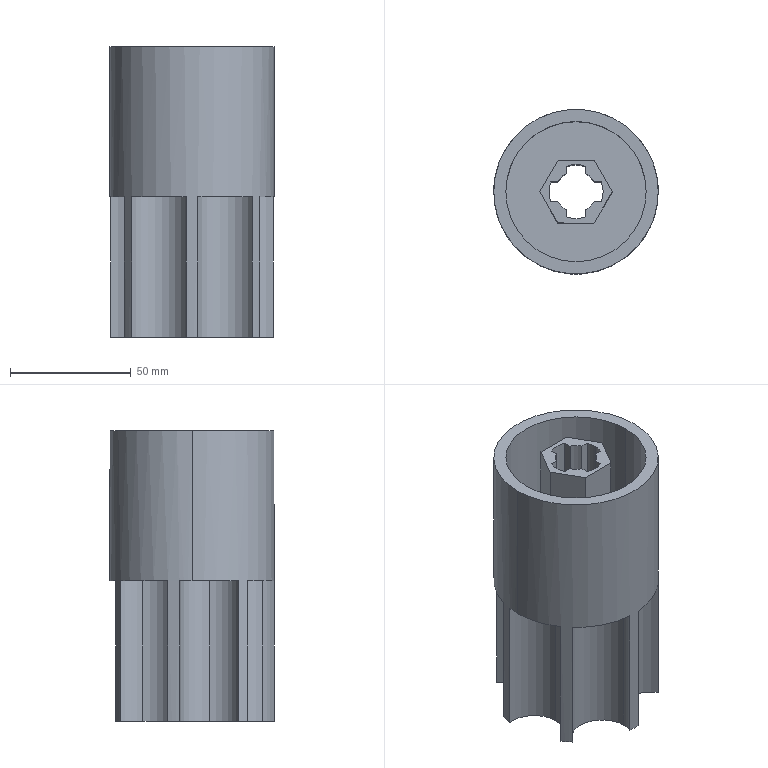Part | SolidWorks | features ICE 2, Extrusion 1 | 1 solid | 48 faces | box 68 x 68 x 120 mm | volume 167321 mm3 | plane 25 | cylinder 23 | commonest cylinder face diameters 25.067 x10 22.4 x5 17 x4 58 x2 68 x2
STEP:
#1=CARTESIAN_POINT('',(11.2,0.,-60.));
#2=VERTEX_POINT('',#1);
#3=CARTESIAN_POINT('',(10.461,4.,-60.));
#4=VERTEX_POINT('',#3);
#5=CARTESIAN_POINT('',(0.,0.,-60.));
#6=DIRECTION('',(0.,0.,1.));
#7=DIRECTION('',(1.,0.,0.));
#8=AXIS2_PLACEMENT_3D('',#5,#6,#7);
#9=CIRCLE('',#8,11.2);
#10=EDGE_CURVE('',#2,#4,#9,.T.);
#11=ORIENTED_EDGE('',*,*,#10,.F.);
#12=CARTESIAN_POINT('',(11.2,0.,60.));
#13=VERTEX_POINT('',#12);
#14=CARTESIAN_POINT('',(11.2,0.,-60.));
#15=DIRECTION('',(0.,0.,1.));
#16=VECTOR('',#15,1000.);
#17=LINE('',#14,#16);
#18=EDGE_CURVE('',#2,#13,#17,.T.);
#19=ORIENTED_EDGE('',*,*,#18,.T.);
#20=CARTESIAN_POINT('',(10.461,4.,60.));
#21=VERTEX_POINT('',#20);
#22=CARTESIAN_POINT('',(0.,0.,60.));
#23=DIRECTION('',(0.,0.,1.));
#24=DIRECTION('',(1.,0.,0.));
#25=AXIS2_PLACEMENT_3D('',#22,#23,#24);
#26=CIRCLE('',#25,11.2);
#27=EDGE_CURVE('',#13,#21,#26,.T.);
#28=ORIENTED_EDGE('',*,*,#27,.T.);
#29=CARTESIAN_POINT('',(10.461,4.,-60.));
#30=DIRECTION('',(0.,0.,1.));
#31=VECTOR('',#30,1000.);
#32=LINE('',#29,#31);
#33=EDGE_CURVE('',#4,#21,#32,.T.);
#34=ORIENTED_EDGE('',*,*,#33,.F.);
#35=EDGE_LOOP('',(#11,#19,#28,#34));
#36=FACE_OUTER_BOUND('',#35,.T.);
#37=CARTESIAN_POINT('',(0.,0.,-60.));
#38=DIRECTION('',(0.,0.,1.));
#39=DIRECTION('',(1.,0.,0.));
#40=AXIS2_PLACEMENT_3D('',#37,#38,#39);
#41=CYLINDRICAL_SURFACE('',#40,11.2);
#42=ADVANCED_FACE('',(#36),#41,.F.);
#43=CARTESIAN_POINT('',(34.,0.,60.));
#44=VERTEX_POINT('',#43);
#45=CARTESIAN_POINT('',(-34.,0.,60.));
#46=VERTEX_POINT('',#45);
#47=CARTESIAN_POINT('',(0.,0.,60.));
#48=DIRECTION('',(0.,0.,1.));
#49=DIRECTION('',(1.,0.,0.));
#50=AXIS2_PLACEMENT_3D('',#47,#48,#49);
#51=CIRCLE('',#50,34.);
#52=EDGE_CURVE('',#44,#46,#51,.T.);
#53=ORIENTED_EDGE('',*,*,#52,.F.);
#54=CARTESIAN_POINT('',(34.,0.,-2.));
#55=VERTEX_POINT('',#54);
#56=CARTESIAN_POINT('',(34.,0.,60.));
#57=DIRECTION('',(0.,0.,-1.));
#58=VECTOR('',#57,1000.);
#59=LINE('',#56,#58);
#60=EDGE_CURVE('',#44,#55,#59,.T.);
#61=ORIENTED_EDGE('',*,*,#60,.T.);
#62=CARTESIAN_POINT('',(33.608,5.151,-2.));
#63=VERTEX_POINT('',#62);
#64=CARTESIAN_POINT('',(0.,0.,-2.));
#65=DIRECTION('',(0.,0.,1.));
#66=DIRECTION('',(1.,0.,0.));
#67=AXIS2_PLACEMENT_3D('',#64,#65,#66);
#68=CIRCLE('',#67,34.);
#69=EDGE_CURVE('',#55,#63,#68,.T.);
#70=ORIENTED_EDGE('',*,*,#69,.T.);
#71=CARTESIAN_POINT('',(33.608,5.151,-60.));
#72=VERTEX_POINT('',#71);
#73=CARTESIAN_POINT('',(33.608,5.151,-60.));
#74=DIRECTION('',(0.,0.,1.));
#75=VECTOR('',#74,1000.);
#76=LINE('',#73,#75);
#77=EDGE_CURVE('',#72,#63,#76,.T.);
#78=ORIENTED_EDGE('',*,*,#77,.F.);
#79=CARTESIAN_POINT('',(32.514,9.941,-60.));
#80=VERTEX_POINT('',#79);
#81=CARTESIAN_POINT('',(0.,0.,-60.));
#82=DIRECTION('',(0.,0.,1.));
#83=DIRECTION('',(1.,0.,0.));
#84=AXIS2_PLACEMENT_3D('',#81,#82,#83);
#85=CIRCLE('',#84,34.);
#86=EDGE_CURVE('',#72,#80,#85,.T.);
#87=ORIENTED_EDGE('',*,*,#86,.T.);
#88=CARTESIAN_POINT('',(32.514,9.941,-2.));
#89=VERTEX_POINT('',#88);
#90=CARTESIAN_POINT('',(32.514,9.941,-60.));
#91=DIRECTION('',(0.,0.,1.));
#92=VECTOR('',#91,1000.);
#93=LINE('',#90,#92);
#94=EDGE_CURVE('',#80,#89,#93,.T.);
#95=ORIENTED_EDGE('',*,*,#94,.T.);
#96=CARTESIAN_POINT('',(16.927,29.487,-2.));
#97=VERTEX_POINT('',#96);
#98=CARTESIAN_POINT('',(0.,0.,-2.));
#99=DIRECTION('',(0.,0.,1.));
#100=DIRECTION('',(1.,0.,0.));
#101=AXIS2_PLACEMENT_3D('',#98,#99,#100);
#102=CIRCLE('',#101,34.);
#103=EDGE_CURVE('',#89,#97,#102,.T.);
#104=ORIENTED_EDGE('',*,*,#103,.T.);
#105=CARTESIAN_POINT('',(16.927,29.487,-60.));
#106=VERTEX_POINT('',#105);
#107=CARTESIAN_POINT('',(16.927,29.487,-60.));
#108=DIRECTION('',(0.,0.,1.));
#109=VECTOR('',#108,1000.);
#110=LINE('',#107,#109);
#111=EDGE_CURVE('',#106,#97,#110,.T.);
#112=ORIENTED_EDGE('',*,*,#111,.F.);
#113=CARTESIAN_POINT('',(12.5,31.619,-60.));
#114=VERTEX_POINT('',#113);
#115=CARTESIAN_POINT('',(0.,0.,-60.));
#116=DIRECTION('',(0.,0.,1.));
#117=DIRECTION('',(1.,0.,0.));
#118=AXIS2_PLACEMENT_3D('',#115,#116,#117);
#119=CIRCLE('',#118,34.);
#120=EDGE_CURVE('',#106,#114,#119,.T.);
#121=ORIENTED_EDGE('',*,*,#120,.T.);
#122=CARTESIAN_POINT('',(12.5,31.619,-2.));
#123=VERTEX_POINT('',#122);
#124=CARTESIAN_POINT('',(12.5,31.619,-60.));
#125=DIRECTION('',(0.,0.,1.));
#126=VECTOR('',#125,1000.);
#127=LINE('',#124,#126);
#128=EDGE_CURVE('',#114,#123,#127,.T.);
#129=ORIENTED_EDGE('',*,*,#128,.T.);
#130=CARTESIAN_POINT('',(-12.5,31.619,-2.));
#131=VERTEX_POINT('',#130);
#132=CARTESIAN_POINT('',(0.,0.,-2.));
#133=DIRECTION('',(0.,0.,1.));
#134=DIRECTION('',(1.,0.,0.));
#135=AXIS2_PLACEMENT_3D('',#132,#133,#134);
#136=CIRCLE('',#135,34.);
#137=EDGE_CURVE('',#123,#131,#136,.T.);
#138=ORIENTED_EDGE('',*,*,#137,.T.);
#139=CARTESIAN_POINT('',(-12.5,31.619,-60.));
#140=VERTEX_POINT('',#139);
#141=CARTESIAN_POINT('',(-12.5,31.619,-60.));
#142=DIRECTION('',(0.,0.,1.));
#143=VECTOR('',#142,1000.);
#144=LINE('',#141,#143);
#145=EDGE_CURVE('',#140,#131,#144,.T.);
#146=ORIENTED_EDGE('',*,*,#145,.F.);
#147=CARTESIAN_POINT('',(-16.927,29.487,-60.));
#148=VERTEX_POINT('',#147);
#149=CARTESIAN_POINT('',(0.,0.,-60.));
#150=DIRECTION('',(0.,0.,1.));
#151=DIRECTION('',(1.,0.,0.));
#152=AXIS2_PLACEMENT_3D('',#149,#150,#151);
#153=CIRCLE('',#152,34.);
#154=EDGE_CURVE('',#140,#148,#153,.T.);
#155=ORIENTED_EDGE('',*,*,#154,.T.);
#156=CARTESIAN_POINT('',(-16.927,29.487,-2.));
#157=VERTEX_POINT('',#156);
#158=CARTESIAN_POINT('',(-16.927,29.487,-60.));
#159=DIRECTION('',(0.,0.,1.));
#160=VECTOR('',#159,1000.);
#161=LINE('',#158,#160);
#162=EDGE_CURVE('',#148,#157,#161,.T.);
#163=ORIENTED_EDGE('',*,*,#162,.T.);
#164=CARTESIAN_POINT('',(-32.514,9.941,-2.));
#165=VERTEX_POINT('',#164);
#166=CARTESIAN_POINT('',(0.,0.,-2.));
#167=DIRECTION('',(0.,0.,1.));
#168=DIRECTION('',(1.,0.,0.));
#169=AXIS2_PLACEMENT_3D('',#166,#167,#168);
#170=CIRCLE('',#169,34.);
#171=EDGE_CURVE('',#157,#165,#170,.T.);
#172=ORIENTED_EDGE('',*,*,#171,.T.);
#173=CARTESIAN_POINT('',(-32.514,9.941,-60.));
#174=VERTEX_POINT('',#173);
#175=CARTESIAN_POINT('',(-32.514,9.941,-60.));
#176=DIRECTION('',(0.,0.,1.));
#177=VECTOR('',#176,1000.);
#178=LINE('',#175,#177);
#179=EDGE_CURVE('',#174,#165,#178,.T.);
#180=ORIENTED_EDGE('',*,*,#179,.F.);
#181=CARTESIAN_POINT('',(-33.608,5.151,-60.));
#182=VERTEX_POINT('',#181);
#183=CARTESIAN_POINT('',(0.,0.,-60.));
#184=DIRECTION('',(0.,0.,1.));
#185=DIRECTION('',(1.,0.,0.));
#186=AXIS2_PLACEMENT_3D('',#183,#184,#185);
#187=CIRCLE('',#186,34.);
#188=EDGE_CURVE('',#174,#182,#187,.T.);
#189=ORIENTED_EDGE('',*,*,#188,.T.);
#190=CARTESIAN_POINT('',(-33.608,5.151,-2.));
#191=VERTEX_POINT('',#190);
#192=CARTESIAN_POINT('',(-33.608,5.151,-60.));
#193=DIRECTION('',(0.,0.,1.));
#194=VECTOR('',#193,1000.);
#195=LINE('',#192,#194);
#196=EDGE_CURVE('',#182,#191,#195,.T.);
#197=ORIENTED_EDGE('',*,*,#196,.T.);
#198=CARTESIAN_POINT('',(-34.,0.,-2.));
#199=VERTEX_POINT('',#198);
#200=CARTESIAN_POINT('',(0.,0.,-2.));
#201=DIRECTION('',(0.,0.,1.));
#202=DIRECTION('',(1.,0.,0.));
#203=AXIS2_PLACEMENT_3D('',#200,#201,#202);
#204=CIRCLE('',#203,34.);
#205=EDGE_CURVE('',#191,#199,#204,.T.);
#206=ORIENTED_EDGE('',*,*,#205,.T.);
#207=CARTESIAN_POINT('',(-34.,0.,60.));
#208=DIRECTION('',(0.,0.,-1.));
#209=VECTOR('',#208,1000.);
#210=LINE('',#207,#209);
#211=EDGE_CURVE('',#46,#199,#210,.T.);
#212=ORIENTED_EDGE('',*,*,#211,.F.);
#213=EDGE_LOOP('',(#53,#61,#70,#78,#87,#95,#104,#112,#121,#129,#138,#146,#155,#163,#172,#180,#189,#197,#206,#212));
#214=FACE_OUTER_BOUND('',#213,.T.);
#215=CARTESIAN_POINT('',(0.,0.,60.));
#216=DIRECTION('',(0.,0.,-1.));
#217=DIRECTION('',(-1.,0.,0.));
#218=AXIS2_PLACEMENT_3D('',#215,#216,#217);
#219=CYLINDRICAL_SURFACE('',#218,34.);
#220=ADVANCED_FACE('',(#214),#219,.T.);
#221=CARTESIAN_POINT('',(-29.,0.,60.));
#222=VERTEX_POINT('',#221);
#223=CARTESIAN_POINT('',(29.,0.,60.));
#224=VERTEX_POINT('',#223);
#225=CARTESIAN_POINT('',(0.,0.,60.));
#226=DIRECTION('',(0.,0.,1.));
#227=DIRECTION('',(1.,0.,0.));
#228=AXIS2_PLACEMENT_3D('',#225,#226,#227);
#229=CIRCLE('',#228,29.);
#230=EDGE_CURVE('',#222,#224,#229,.T.);
#231=ORIENTED_EDGE('',*,*,#230,.T.);
#232=CARTESIAN_POINT('',(29.,0.,0.));
#233=VERTEX_POINT('',#232);
#234=CARTESIAN_POINT('',(29.,0.,60.));
#235=DIRECTION('',(0.,0.,-1.));
#236=VECTOR('',#235,1000.);
#237=LINE('',#234,#236);
#238=EDGE_CURVE('',#224,#233,#237,.T.);
#239=ORIENTED_EDGE('',*,*,#238,.T.);
#240=CARTESIAN_POINT('',(-29.,0.,0.));
#241=VERTEX_POINT('',#240);
#242=CARTESIAN_POINT('',(0.,0.,0.));
#243=DIRECTION('',(0.,0.,1.));
#244=DIRECTION('',(1.,0.,0.));
#245=AXIS2_PLACEMENT_3D('',#242,#243,#244);
#246=CIRCLE('',#245,29.);
#247=EDGE_CURVE('',#241,#233,#246,.T.);
#248=ORIENTED_EDGE('',*,*,#247,.F.);
#249=CARTESIAN_POINT('',(-29.,0.,60.));
#250=DIRECTION('',(0.,0.,-1.));
#251=VECTOR('',#250,1000.);
#252=LINE('',#249,#251);
#253=EDGE_CURVE('',#222,#241,#252,.T.);
#254=ORIENTED_EDGE('',*,*,#253,.F.);
#255=EDGE_LOOP('',(#231,#239,#248,#254));
#256=FACE_OUTER_BOUND('',#255,.T.);
#257=CARTESIAN_POINT('',(0.,0.,60.));
#258=DIRECTION('',(0.,0.,-1.));
#259=DIRECTION('',(-1.,0.,0.));
#260=AXIS2_PLACEMENT_3D('',#257,#258,#259);
#261=CYLINDRICAL_SURFACE('',#260,29.);
#262=ADVANCED_FACE('',(#256),#261,.F.);
#263=CARTESIAN_POINT('',(-12.902,20.284,-60.));
#264=VERTEX_POINT('',#263);
#265=CARTESIAN_POINT('',(-25.436,20.284,-60.));
#266=DIRECTION('',(0.,0.,-1.));
#267=DIRECTION('',(-1.,0.,0.));
#268=AXIS2_PLACEMENT_3D('',#265,#266,#267);
#269=CIRCLE('',#268,12.533);
#270=EDGE_CURVE('',#148,#264,#269,.T.);
#271=ORIENTED_EDGE('',*,*,#270,.T.);
#272=CARTESIAN_POINT('',(-12.902,20.284,-2.));
#273=VERTEX_POINT('',#272);
#274=CARTESIAN_POINT('',(-12.902,20.284,-60.));
#275=DIRECTION('',(0.,0.,1.));
#276=VECTOR('',#275,1000.);
#277=LINE('',#274,#276);
#278=EDGE_CURVE('',#264,#273,#277,.T.);
#279=ORIENTED_EDGE('',*,*,#278,.T.);
#280=CARTESIAN_POINT('',(-25.436,20.284,-2.));
#281=DIRECTION('',(0.,0.,1.));
#282=DIRECTION('',(1.,0.,0.));
#283=AXIS2_PLACEMENT_3D('',#280,#281,#282);
#284=CIRCLE('',#283,12.533);
#285=EDGE_CURVE('',#273,#157,#284,.T.);
#286=ORIENTED_EDGE('',*,*,#285,.T.);
#287=ORIENTED_EDGE('',*,*,#162,.F.);
#288=EDGE_LOOP('',(#271,#279,#286,#287));
#289=FACE_OUTER_BOUND('',#288,.T.);
#290=CARTESIAN_POINT('',(-25.436,20.284,-60.));
#291=DIRECTION('',(0.,0.,1.));
#292=DIRECTION('',(1.,0.,0.));
#293=AXIS2_PLACEMENT_3D('',#290,#291,#292);
#294=CYLINDRICAL_SURFACE('',#293,12.533);
#295=ADVANCED_FACE('',(#289),#294,.F.);
#296=CARTESIAN_POINT('',(-19.184,-7.239,-60.));
#297=VERTEX_POINT('',#296);
#298=CARTESIAN_POINT('',(-31.718,-7.239,-60.));
#299=DIRECTION('',(0.,0.,-1.));
#300=DIRECTION('',(-1.,0.,0.));
#301=AXIS2_PLACEMENT_3D('',#298,#299,#300);
#302=CIRCLE('',#301,12.533);
#303=EDGE_CURVE('',#182,#297,#302,.T.);
#304=ORIENTED_EDGE('',*,*,#303,.T.);
#305=CARTESIAN_POINT('',(-19.184,-7.239,-2.));
#306=VERTEX_POINT('',#305);
#307=CARTESIAN_POINT('',(-19.184,-7.239,-60.));
#308=DIRECTION('',(0.,0.,1.));
#309=VECTOR('',#308,1000.);
#310=LINE('',#307,#309);
#311=EDGE_CURVE('',#297,#306,#310,.T.);
#312=ORIENTED_EDGE('',*,*,#311,.T.);
#313=CARTESIAN_POINT('',(-31.718,-7.239,-2.));
#314=DIRECTION('',(0.,0.,1.));
#315=DIRECTION('',(1.,0.,0.));
#316=AXIS2_PLACEMENT_3D('',#313,#314,#315);
#317=CIRCLE('',#316,12.533);
#318=EDGE_CURVE('',#306,#191,#317,.T.);
#319=ORIENTED_EDGE('',*,*,#318,.T.);
#320=ORIENTED_EDGE('',*,*,#196,.F.);
#321=EDGE_LOOP('',(#304,#312,#319,#320));
#322=FACE_OUTER_BOUND('',#321,.T.);
#323=CARTESIAN_POINT('',(-31.718,-7.239,-60.));
#324=DIRECTION('',(0.,0.,1.));
#325=DIRECTION('',(1.,0.,0.));
#326=AXIS2_PLACEMENT_3D('',#323,#324,#325);
#327=CYLINDRICAL_SURFACE('',#326,12.533);
#328=ADVANCED_FACE('',(#322),#327,.F.);
#329=CARTESIAN_POINT('',(-24.981,-23.064,-60.));
#330=VERTEX_POINT('',#329);
#331=CARTESIAN_POINT('',(-1.582,-29.312,-60.));
#332=VERTEX_POINT('',#331);
#333=CARTESIAN_POINT('',(-14.116,-29.312,-60.));
#334=DIRECTION('',(0.,0.,-1.));
#335=DIRECTION('',(-1.,0.,0.));
#336=AXIS2_PLACEMENT_3D('',#333,#334,#335);
#337=CIRCLE('',#336,12.533);
#338=EDGE_CURVE('',#330,#332,#337,.T.);
#339=ORIENTED_EDGE('',*,*,#338,.T.);
#340=CARTESIAN_POINT('',(-1.582,-29.312,-2.));
#341=VERTEX_POINT('',#340);
#342=CARTESIAN_POINT('',(-1.582,-29.312,-60.));
#343=DIRECTION('',(0.,0.,1.));
#344=VECTOR('',#343,1000.);
#345=LINE('',#342,#344);
#346=EDGE_CURVE('',#332,#341,#345,.T.);
#347=ORIENTED_EDGE('',*,*,#346,.T.);
#348=CARTESIAN_POINT('',(-24.981,-23.064,-2.));
#349=VERTEX_POINT('',#348);
#350=CARTESIAN_POINT('',(-14.116,-29.312,-2.));
#351=DIRECTION('',(0.,0.,1.));
#352=DIRECTION('',(1.,0.,0.));
#353=AXIS2_PLACEMENT_3D('',#350,#351,#352);
#354=CIRCLE('',#353,12.533);
#355=EDGE_CURVE('',#341,#349,#354,.T.);
#356=ORIENTED_EDGE('',*,*,#355,.T.);
#357=CARTESIAN_POINT('',(-24.981,-23.064,-60.));
#358=DIRECTION('',(0.,0.,1.));
#359=VECTOR('',#358,1000.);
#360=LINE('',#357,#359);
#361=EDGE_CURVE('',#330,#349,#360,.T.);
#362=ORIENTED_EDGE('',*,*,#361,.F.);
#363=EDGE_LOOP('',(#339,#347,#356,#362));
#364=FACE_OUTER_BOUND('',#363,.T.);
#365=CARTESIAN_POINT('',(-14.116,-29.312,-60.));
#366=DIRECTION('',(0.,0.,1.));
#367=DIRECTION('',(1.,0.,0.));
#368=AXIS2_PLACEMENT_3D('',#365,#366,#367);
#369=CYLINDRICAL_SURFACE('',#368,12.533);
#370=ADVANCED_FACE('',(#364),#369,.F.);
#371=ORIENTED_EDGE('',*,*,#145,.T.);
#372=CARTESIAN_POINT('',(0.,32.533,-2.));
#373=DIRECTION('',(0.,0.,1.));
#374=DIRECTION('',(1.,0.,0.));
#375=AXIS2_PLACEMENT_3D('',#372,#373,#374);
#376=CIRCLE('',#375,12.533);
#377=EDGE_CURVE('',#131,#123,#376,.T.);
#378=ORIENTED_EDGE('',*,*,#377,.T.);
#379=ORIENTED_EDGE('',*,*,#128,.F.);
#380=CARTESIAN_POINT('',(0.,32.533,-60.));
#381=DIRECTION('',(0.,0.,-1.));
#382=DIRECTION('',(-1.,0.,0.));
#383=AXIS2_PLACEMENT_3D('',#380,#381,#382);
#384=CIRCLE('',#383,12.533);
#385=EDGE_CURVE('',#114,#140,#384,.T.);
#386=ORIENTED_EDGE('',*,*,#385,.T.);
#387=EDGE_LOOP('',(#371,#378,#379,#386));
#388=FACE_OUTER_BOUND('',#387,.T.);
#389=CARTESIAN_POINT('',(0.,32.533,-60.));
#390=DIRECTION('',(0.,0.,1.));
#391=DIRECTION('',(1.,0.,0.));
#392=AXIS2_PLACEMENT_3D('',#389,#390,#391);
#393=CYLINDRICAL_SURFACE('',#392,12.533);
#394=ADVANCED_FACE('',(#388),#393,.F.);
#395=ORIENTED_EDGE('',*,*,#111,.T.);
#396=CARTESIAN_POINT('',(25.436,20.284,-2.));
#397=DIRECTION('',(0.,0.,1.));
#398=DIRECTION('',(1.,0.,0.));
#399=AXIS2_PLACEMENT_3D('',#396,#397,#398);
#400=CIRCLE('',#399,12.533);
#401=EDGE_CURVE('',#97,#89,#400,.T.);
#402=ORIENTED_EDGE('',*,*,#401,.T.);
#403=ORIENTED_EDGE('',*,*,#94,.F.);
#404=CARTESIAN_POINT('',(25.436,20.284,-60.));
#405=DIRECTION('',(0.,0.,-1.));
#406=DIRECTION('',(-1.,0.,0.));
#407=AXIS2_PLACEMENT_3D('',#404,#405,#406);
#408=CIRCLE('',#407,12.533);
#409=EDGE_CURVE('',#80,#106,#408,.T.);
#410=ORIENTED_EDGE('',*,*,#409,.T.);
#411=EDGE_LOOP('',(#395,#402,#403,#410));
#412=FACE_OUTER_BOUND('',#411,.T.);
#413=CARTESIAN_POINT('',(25.436,20.284,-60.));
#414=DIRECTION('',(0.,0.,1.));
#415=DIRECTION('',(1.,0.,0.));
#416=AXIS2_PLACEMENT_3D('',#413,#414,#415);
#417=CYLINDRICAL_SURFACE('',#416,12.533);
#418=ADVANCED_FACE('',(#412),#417,.F.);
#419=ORIENTED_EDGE('',*,*,#77,.T.);
#420=CARTESIAN_POINT('',(28.045,-19.222,-2.));
#421=VERTEX_POINT('',#420);
#422=CARTESIAN_POINT('',(31.718,-7.239,-2.));
#423=DIRECTION('',(0.,0.,1.));
#424=DIRECTION('',(1.,0.,0.));
#425=AXIS2_PLACEMENT_3D('',#422,#423,#424);
#426=CIRCLE('',#425,12.533);
#427=EDGE_CURVE('',#63,#421,#426,.T.);
#428=ORIENTED_EDGE('',*,*,#427,.T.);
#429=CARTESIAN_POINT('',(28.045,-19.222,-60.));
#430=VERTEX_POINT('',#429);
#431=CARTESIAN_POINT('',(28.045,-19.222,-60.));
#432=DIRECTION('',(0.,0.,1.));
#433=VECTOR('',#432,1000.);
#434=LINE('',#431,#433);
#435=EDGE_CURVE('',#430,#421,#434,.T.);
#436=ORIENTED_EDGE('',*,*,#435,.F.);
#437=CARTESIAN_POINT('',(31.718,-7.239,-60.));
#438=DIRECTION('',(0.,0.,-1.));
#439=DIRECTION('',(-1.,0.,0.));
#440=AXIS2_PLACEMENT_3D('',#437,#438,#439);
#441=CIRCLE('',#440,12.533);
#442=EDGE_CURVE('',#430,#72,#441,.T.);
#443=ORIENTED_EDGE('',*,*,#442,.T.);
#444=EDGE_LOOP('',(#419,#428,#436,#443));
#445=FACE_OUTER_BOUND('',#444,.T.);
#446=CARTESIAN_POINT('',(31.718,-7.239,-60.));
#447=DIRECTION('',(0.,0.,1.));
#448=DIRECTION('',(1.,0.,0.));
#449=AXIS2_PLACEMENT_3D('',#446,#447,#448);
#450=CYLINDRICAL_SURFACE('',#449,12.533);
#451=ADVANCED_FACE('',(#445),#450,.F.);
#452=CARTESIAN_POINT('',(24.981,-23.064,-60.));
#453=VERTEX_POINT('',#452);
#454=CARTESIAN_POINT('',(24.981,-23.064,-2.));
#455=VERTEX_POINT('',#454);
#456=CARTESIAN_POINT('',(24.981,-23.064,-60.));
#457=DIRECTION('',(0.,0.,1.));
#458=VECTOR('',#457,1000.);
#459=LINE('',#456,#458);
#460=EDGE_CURVE('',#453,#455,#459,.T.);
#461=ORIENTED_EDGE('',*,*,#460,.T.);
#462=CARTESIAN_POINT('',(2.457,-33.911,-2.));
#463=VERTEX_POINT('',#462);
#464=CARTESIAN_POINT('',(14.116,-29.312,-2.));
#465=DIRECTION('',(0.,0.,1.));
#466=DIRECTION('',(1.,0.,0.));
#467=AXIS2_PLACEMENT_3D('',#464,#465,#466);
#468=CIRCLE('',#467,12.533);
#469=EDGE_CURVE('',#455,#463,#468,.T.);
#470=ORIENTED_EDGE('',*,*,#469,.T.);
#471=CARTESIAN_POINT('',(2.457,-33.911,-60.));
#472=VERTEX_POINT('',#471);
#473=CARTESIAN_POINT('',(2.457,-33.911,-60.));
#474=DIRECTION('',(0.,0.,1.));
#475=VECTOR('',#474,1000.);
#476=LINE('',#473,#475);
#477=EDGE_CURVE('',#472,#463,#476,.T.);
#478=ORIENTED_EDGE('',*,*,#477,.F.);
#479=CARTESIAN_POINT('',(14.116,-29.312,-60.));
#480=DIRECTION('',(0.,0.,-1.));
#481=DIRECTION('',(-1.,0.,0.));
#482=AXIS2_PLACEMENT_3D('',#479,#480,#481);
#483=CIRCLE('',#482,12.533);
#484=EDGE_CURVE('',#472,#453,#483,.T.);
#485=ORIENTED_EDGE('',*,*,#484,.T.);
#486=EDGE_LOOP('',(#461,#470,#478,#485));
#487=FACE_OUTER_BOUND('',#486,.T.);
#488=CARTESIAN_POINT('',(14.116,-29.312,-60.));
#489=DIRECTION('',(0.,0.,1.));
#490=DIRECTION('',(1.,0.,0.));
#491=AXIS2_PLACEMENT_3D('',#488,#489,#490);
#492=CYLINDRICAL_SURFACE('',#491,12.533);
#493=ADVANCED_FACE('',(#487),#492,.F.);
#494=ORIENTED_EDGE('',*,*,#346,.F.);
#495=CARTESIAN_POINT('',(-2.457,-33.911,-60.));
#496=VERTEX_POINT('',#495);
#497=CARTESIAN_POINT('',(-14.116,-29.312,-60.));
#498=DIRECTION('',(0.,0.,-1.));
#499=DIRECTION('',(-1.,0.,0.));
#500=AXIS2_PLACEMENT_3D('',#497,#498,#499);
#501=CIRCLE('',#500,12.533);
#502=EDGE_CURVE('',#332,#496,#501,.T.);
#503=ORIENTED_EDGE('',*,*,#502,.T.);
#504=CARTESIAN_POINT('',(-2.457,-33.911,-2.));
#505=VERTEX_POINT('',#504);
#506=CARTESIAN_POINT('',(-2.457,-33.911,-60.));
#507=DIRECTION('',(0.,0.,1.));
#508=VECTOR('',#507,1000.);
#509=LINE('',#506,#508);
#510=EDGE_CURVE('',#496,#505,#509,.T.);
#511=ORIENTED_EDGE('',*,*,#510,.T.);
#512=CARTESIAN_POINT('',(-14.116,-29.312,-2.));
#513=DIRECTION('',(0.,0.,1.));
#514=DIRECTION('',(1.,0.,0.));
#515=AXIS2_PLACEMENT_3D('',#512,#513,#514);
#516=CIRCLE('',#515,12.533);
#517=EDGE_CURVE('',#505,#341,#516,.T.);
#518=ORIENTED_EDGE('',*,*,#517,.T.);
#519=EDGE_LOOP('',(#494,#503,#511,#518));
#520=FACE_OUTER_BOUND('',#519,.T.);
#521=CARTESIAN_POINT('',(-14.116,-29.312,-60.));
#522=DIRECTION('',(0.,0.,1.));
#523=DIRECTION('',(1.,0.,0.));
#524=AXIS2_PLACEMENT_3D('',#521,#522,#523);
#525=CYLINDRICAL_SURFACE('',#524,12.533);
#526=ADVANCED_FACE('',(#520),#525,.F.);
#527=ORIENTED_EDGE('',*,*,#311,.F.);
#528=CARTESIAN_POINT('',(-28.045,-19.222,-60.));
#529=VERTEX_POINT('',#528);
#530=CARTESIAN_POINT('',(-31.718,-7.239,-60.));
#531=DIRECTION('',(0.,0.,-1.));
#532=DIRECTION('',(-1.,0.,0.));
#533=AXIS2_PLACEMENT_3D('',#530,#531,#532);
#534=CIRCLE('',#533,12.533);
#535=EDGE_CURVE('',#297,#529,#534,.T.);
#536=ORIENTED_EDGE('',*,*,#535,.T.);
#537=CARTESIAN_POINT('',(-28.045,-19.222,-2.));
#538=VERTEX_POINT('',#537);
#539=CARTESIAN_POINT('',(-28.045,-19.222,-60.));
#540=DIRECTION('',(0.,0.,1.));
#541=VECTOR('',#540,1000.);
#542=LINE('',#539,#541);
#543=EDGE_CURVE('',#529,#538,#542,.T.);
#544=ORIENTED_EDGE('',*,*,#543,.T.);
#545=CARTESIAN_POINT('',(-31.718,-7.239,-2.));
#546=DIRECTION('',(0.,0.,1.));
#547=DIRECTION('',(1.,0.,0.));
#548=AXIS2_PLACEMENT_3D('',#545,#546,#547);
#549=CIRCLE('',#548,12.533);
#550=EDGE_CURVE('',#538,#306,#549,.T.);
#551=ORIENTED_EDGE('',*,*,#550,.T.);
#552=EDGE_LOOP('',(#527,#536,#544,#551));
#553=FACE_OUTER_BOUND('',#552,.T.);
#554=CARTESIAN_POINT('',(-31.718,-7.239,-60.));
#555=DIRECTION('',(0.,0.,1.));
#556=DIRECTION('',(1.,0.,0.));
#557=AXIS2_PLACEMENT_3D('',#554,#555,#556);
#558=CYLINDRICAL_SURFACE('',#557,12.533);
#559=ADVANCED_FACE('',(#553),#558,.F.);
#560=ORIENTED_EDGE('',*,*,#278,.F.);
#561=CARTESIAN_POINT('',(-25.436,20.284,-60.));
#562=DIRECTION('',(0.,0.,-1.));
#563=DIRECTION('',(-1.,0.,0.));
#564=AXIS2_PLACEMENT_3D('',#561,#562,#563);
#565=CIRCLE('',#564,12.533);
#566=EDGE_CURVE('',#264,#174,#565,.T.);
#567=ORIENTED_EDGE('',*,*,#566,.T.);
#568=ORIENTED_EDGE('',*,*,#179,.T.);
#569=CARTESIAN_POINT('',(-25.436,20.284,-2.));
#570=DIRECTION('',(0.,0.,1.));
#571=DIRECTION('',(1.,0.,0.));
#572=AXIS2_PLACEMENT_3D('',#569,#570,#571);
#573=CIRCLE('',#572,12.533);
#574=EDGE_CURVE('',#165,#273,#573,.T.);
#575=ORIENTED_EDGE('',*,*,#574,.T.);
#576=EDGE_LOOP('',(#560,#567,#568,#575));
#577=FACE_OUTER_BOUND('',#576,.T.);
#578=CARTESIAN_POINT('',(-25.436,20.284,-60.));
#579=DIRECTION('',(0.,0.,1.));
#580=DIRECTION('',(1.,0.,0.));
#581=AXIS2_PLACEMENT_3D('',#578,#579,#580);
#582=CYLINDRICAL_SURFACE('',#581,12.533);
#583=ADVANCED_FACE('',(#577),#582,.F.);
#584=ORIENTED_EDGE('',*,*,#247,.T.);
#585=CARTESIAN_POINT('',(0.,0.,0.));
#586=DIRECTION('',(0.,0.,1.));
#587=DIRECTION('',(1.,0.,0.));
#588=AXIS2_PLACEMENT_3D('',#585,#586,#587);
#589=CIRCLE('',#588,29.);
#590=EDGE_CURVE('',#233,#241,#589,.T.);
#591=ORIENTED_EDGE('',*,*,#590,.T.);
#592=EDGE_LOOP('',(#584,#591));
#593=FACE_OUTER_BOUND('',#592,.T.);
#594=CARTESIAN_POINT('',(-15.,0.07819,0.));
#595=VERTEX_POINT('',#594);
#596=CARTESIAN_POINT('',(-7.568,-12.951,0.));
#597=VERTEX_POINT('',#596);
#598=CARTESIAN_POINT('',(20.97,-62.98,0.));
#599=DIRECTION('',(0.4955,-0.8686,0.));
#600=VECTOR('',#599,1000.);
#601=LINE('',#598,#600);
#602=EDGE_CURVE('',#595,#597,#601,.T.);
#603=ORIENTED_EDGE('',*,*,#602,.F.);
#604=CARTESIAN_POINT('',(-7.432,13.029,0.));
#605=VERTEX_POINT('',#604);
#606=CARTESIAN_POINT('',(-43.86,-49.313,0.));
#607=DIRECTION('',(-0.5045,-0.8634,0.));
#608=VECTOR('',#607,1000.);
#609=LINE('',#606,#608);
#610=EDGE_CURVE('',#605,#595,#609,.T.);
#611=ORIENTED_EDGE('',*,*,#610,.F.);
#612=CARTESIAN_POINT('',(7.568,12.951,0.));
#613=VERTEX_POINT('',#612);
#614=CARTESIAN_POINT('',(0.4583,12.988,0.));
#615=DIRECTION('',(-1.,0.005212,0.));
#616=VECTOR('',#615,1000.);
#617=LINE('',#614,#616);
#618=EDGE_CURVE('',#613,#605,#617,.T.);
#619=ORIENTED_EDGE('',*,*,#618,.F.);
#620=CARTESIAN_POINT('',(15.,-0.07819,0.));
#621=VERTEX_POINT('',#620);
#622=CARTESIAN_POINT('',(43.537,-50.107,0.));
#623=DIRECTION('',(-0.4955,0.8686,0.));
#624=VECTOR('',#623,1000.);
#625=LINE('',#622,#624);
#626=EDGE_CURVE('',#621,#613,#625,.T.);
#627=ORIENTED_EDGE('',*,*,#626,.F.);
#628=CARTESIAN_POINT('',(7.432,-13.029,0.));
#629=VERTEX_POINT('',#628);
#630=CARTESIAN_POINT('',(-21.428,-62.421,0.));
#631=DIRECTION('',(0.5045,0.8634,0.));
#632=VECTOR('',#631,1000.);
#633=LINE('',#630,#632);
#634=EDGE_CURVE('',#629,#621,#633,.T.);
#635=ORIENTED_EDGE('',*,*,#634,.F.);
#636=CARTESIAN_POINT('',(0.3229,-12.992,0.));
#637=DIRECTION('',(1.,-0.005212,0.));
#638=VECTOR('',#637,1000.);
#639=LINE('',#636,#638);
#640=EDGE_CURVE('',#597,#629,#639,.T.);
#641=ORIENTED_EDGE('',*,*,#640,.F.);
#642=EDGE_LOOP('',(#603,#611,#619,#627,#635,#641));
#643=FACE_BOUND('',#642,.T.);
#644=CARTESIAN_POINT('',(0.,16.267,0.));
#645=DIRECTION('',(0.,0.,-1.));
#646=DIRECTION('',(-1.,0.,0.));
#647=AXIS2_PLACEMENT_3D('',#644,#645,#646);
#648=PLANE('',#647);
#649=ADVANCED_FACE('',(#593,#643),#648,.F.);
#650=ORIENTED_EDGE('',*,*,#238,.F.);
#651=CARTESIAN_POINT('',(0.,0.,60.));
#652=DIRECTION('',(0.,0.,1.));
#653=DIRECTION('',(1.,0.,0.));
#654=AXIS2_PLACEMENT_3D('',#651,#652,#653);
#655=CIRCLE('',#654,29.);
#656=EDGE_CURVE('',#224,#222,#655,.T.);
#657=ORIENTED_EDGE('',*,*,#656,.T.);
#658=ORIENTED_EDGE('',*,*,#253,.T.);
#659=ORIENTED_EDGE('',*,*,#590,.F.);
#660=EDGE_LOOP('',(#650,#657,#658,#659));
#661=FACE_OUTER_BOUND('',#660,.T.);
#662=CARTESIAN_POINT('',(0.,0.,60.));
#663=DIRECTION('',(0.,0.,-1.));
#664=DIRECTION('',(-1.,0.,0.));
#665=AXIS2_PLACEMENT_3D('',#662,#663,#664);
#666=CYLINDRICAL_SURFACE('',#665,29.);
#667=ADVANCED_FACE('',(#661),#666,.F.);
#668=ORIENTED_EDGE('',*,*,#60,.F.);
#669=CARTESIAN_POINT('',(0.,0.,60.));
#670=DIRECTION('',(0.,0.,1.));
#671=DIRECTION('',(1.,0.,0.));
#672=AXIS2_PLACEMENT_3D('',#669,#670,#671);
#673=CIRCLE('',#672,34.);
#674=EDGE_CURVE('',#46,#44,#673,.T.);
#675=ORIENTED_EDGE('',*,*,#674,.F.);
#676=ORIENTED_EDGE('',*,*,#211,.T.);
#677=CARTESIAN_POINT('',(0.,0.,-2.));
#678=DIRECTION('',(0.,0.,1.));
#679=DIRECTION('',(1.,0.,0.));
#680=AXIS2_PLACEMENT_3D('',#677,#678,#679);
#681=CIRCLE('',#680,34.);
#682=EDGE_CURVE('',#199,#538,#681,.T.);
#683=ORIENTED_EDGE('',*,*,#682,.T.);
#684=ORIENTED_EDGE('',*,*,#543,.F.);
#685=CARTESIAN_POINT('',(0.,0.,-60.));
#686=DIRECTION('',(0.,0.,1.));
#687=DIRECTION('',(1.,0.,0.));
#688=AXIS2_PLACEMENT_3D('',#685,#686,#687);
#689=CIRCLE('',#688,34.);
#690=EDGE_CURVE('',#529,#330,#689,.T.);
#691=ORIENTED_EDGE('',*,*,#690,.T.);
#692=ORIENTED_EDGE('',*,*,#361,.T.);
#693=CARTESIAN_POINT('',(0.,0.,-2.));
#694=DIRECTION('',(0.,0.,1.));
#695=DIRECTION('',(1.,0.,0.));
#696=AXIS2_PLACEMENT_3D('',#693,#694,#695);
#697=CIRCLE('',#696,34.);
#698=EDGE_CURVE('',#349,#505,#697,.T.);
#699=ORIENTED_EDGE('',*,*,#698,.T.);
#700=ORIENTED_EDGE('',*,*,#510,.F.);
#701=CARTESIAN_POINT('',(0.,0.,-60.));
#702=DIRECTION('',(0.,0.,1.));
#703=DIRECTION('',(1.,0.,0.));
#704=AXIS2_PLACEMENT_3D('',#701,#702,#703);
#705=CIRCLE('',#704,34.);
#706=EDGE_CURVE('',#496,#472,#705,.T.);
#707=ORIENTED_EDGE('',*,*,#706,.T.);
#708=ORIENTED_EDGE('',*,*,#477,.T.);
#709=CARTESIAN_POINT('',(0.,0.,-2.));
#710=DIRECTION('',(0.,0.,1.));
#711=DIRECTION('',(1.,0.,0.));
#712=AXIS2_PLACEMENT_3D('',#709,#710,#711);
#713=CIRCLE('',#712,34.);
#714=EDGE_CURVE('',#463,#455,#713,.T.);
#715=ORIENTED_EDGE('',*,*,#714,.T.);
#716=ORIENTED_EDGE('',*,*,#460,.F.);
#717=CARTESIAN_POINT('',(0.,0.,-60.));
#718=DIRECTION('',(0.,0.,1.));
#719=DIRECTION('',(1.,0.,0.));
#720=AXIS2_PLACEMENT_3D('',#717,#718,#719);
#721=CIRCLE('',#720,34.);
#722=EDGE_CURVE('',#453,#430,#721,.T.);
#723=ORIENTED_EDGE('',*,*,#722,.T.);
#724=ORIENTED_EDGE('',*,*,#435,.T.);
#725=CARTESIAN_POINT('',(0.,0.,-2.));
#726=DIRECTION('',(0.,0.,1.));
#727=DIRECTION('',(1.,0.,0.));
#728=AXIS2_PLACEMENT_3D('',#725,#726,#727);
#729=CIRCLE('',#728,34.);
#730=EDGE_CURVE('',#421,#55,#729,.T.);
#731=ORIENTED_EDGE('',*,*,#730,.T.);
#732=EDGE_LOOP('',(#668,#675,#676,#683,#684,#691,#692,#699,#700,#707,#708,#715,#716,#723,#724,#731));
#733=FACE_OUTER_BOUND('',#732,.T.);
#734=CARTESIAN_POINT('',(0.,0.,60.));
#735=DIRECTION('',(0.,0.,-1.));
#736=DIRECTION('',(-1.,0.,0.));
#737=AXIS2_PLACEMENT_3D('',#734,#735,#736);
#738=CYLINDRICAL_SURFACE('',#737,34.);
#739=ADVANCED_FACE('',(#733),#738,.T.);
#740=ORIENTED_EDGE('',*,*,#230,.F.);
#741=ORIENTED_EDGE('',*,*,#656,.F.);
#742=EDGE_LOOP('',(#740,#741));
#743=FACE_BOUND('',#742,.T.);
#744=ORIENTED_EDGE('',*,*,#674,.T.);
#745=ORIENTED_EDGE('',*,*,#52,.T.);
#746=EDGE_LOOP('',(#744,#745));
#747=FACE_OUTER_BOUND('',#746,.T.);
#748=CARTESIAN_POINT('',(0.,-74.941,60.));
#749=DIRECTION('',(0.,0.,1.));
#750=DIRECTION('',(1.,0.,0.));
#751=AXIS2_PLACEMENT_3D('',#748,#749,#750);
#752=PLANE('',#751);
#753=ADVANCED_FACE('',(#743,#747),#752,.T.);
#754=CARTESIAN_POINT('',(-7.5,-4.,-60.));
#755=VERTEX_POINT('',#754);
#756=CARTESIAN_POINT('',(-4.,-7.5,-60.));
#757=VERTEX_POINT('',#756);
#758=CARTESIAN_POINT('',(0.,0.,-60.));
#759=DIRECTION('',(0.,0.,1.));
#760=DIRECTION('',(1.,0.,0.));
#761=AXIS2_PLACEMENT_3D('',#758,#759,#760);
#762=CIRCLE('',#761,8.5);
#763=EDGE_CURVE('',#755,#757,#762,.T.);
#764=ORIENTED_EDGE('',*,*,#763,.T.);
#765=CARTESIAN_POINT('',(-4.,-10.461,-60.));
#766=VERTEX_POINT('',#765);
#767=CARTESIAN_POINT('',(-4.,-10.461,-60.));
#768=DIRECTION('',(0.,-1.,0.));
#769=VECTOR('',#768,1000.);
#770=LINE('',#767,#769);
#771=EDGE_CURVE('',#757,#766,#770,.T.);
#772=ORIENTED_EDGE('',*,*,#771,.T.);
#773=CARTESIAN_POINT('',(4.,-10.461,-60.));
#774=VERTEX_POINT('',#773);
#775=CARTESIAN_POINT('',(0.,0.,-60.));
#776=DIRECTION('',(0.,0.,1.));
#777=DIRECTION('',(1.,0.,0.));
#778=AXIS2_PLACEMENT_3D('',#775,#776,#777);
#779=CIRCLE('',#778,11.2);
#780=EDGE_CURVE('',#766,#774,#779,.T.);
#781=ORIENTED_EDGE('',*,*,#780,.T.);
#782=CARTESIAN_POINT('',(4.,-7.5,-60.));
#783=VERTEX_POINT('',#782);
#784=CARTESIAN_POINT('',(4.,-10.461,-60.));
#785=DIRECTION('',(0.,1.,0.));
#786=VECTOR('',#785,1000.);
#787=LINE('',#784,#786);
#788=EDGE_CURVE('',#774,#783,#787,.T.);
#789=ORIENTED_EDGE('',*,*,#788,.T.);
#790=CARTESIAN_POINT('',(7.5,-4.,-60.));
#791=VERTEX_POINT('',#790);
#792=CARTESIAN_POINT('',(0.,0.,-60.));
#793=DIRECTION('',(0.,0.,1.));
#794=DIRECTION('',(1.,0.,0.));
#795=AXIS2_PLACEMENT_3D('',#792,#793,#794);
#796=CIRCLE('',#795,8.5);
#797=EDGE_CURVE('',#783,#791,#796,.T.);
#798=ORIENTED_EDGE('',*,*,#797,.T.);
#799=CARTESIAN_POINT('',(10.461,-4.,-60.));
#800=VERTEX_POINT('',#799);
#801=CARTESIAN_POINT('',(10.461,-4.,-60.));
#802=DIRECTION('',(1.,0.,0.));
#803=VECTOR('',#802,1000.);
#804=LINE('',#801,#803);
#805=EDGE_CURVE('',#791,#800,#804,.T.);
#806=ORIENTED_EDGE('',*,*,#805,.T.);
#807=CARTESIAN_POINT('',(0.,0.,-60.));
#808=DIRECTION('',(0.,0.,1.));
#809=DIRECTION('',(1.,0.,0.));
#810=AXIS2_PLACEMENT_3D('',#807,#808,#809);
#811=CIRCLE('',#810,11.2);
#812=EDGE_CURVE('',#800,#2,#811,.T.);
#813=ORIENTED_EDGE('',*,*,#812,.T.);
#814=ORIENTED_EDGE('',*,*,#10,.T.);
#815=CARTESIAN_POINT('',(7.5,4.,-60.));
#816=VERTEX_POINT('',#815);
#817=CARTESIAN_POINT('',(10.461,4.,-60.));
#818=DIRECTION('',(-1.,0.,0.));
#819=VECTOR('',#818,1000.);
#820=LINE('',#817,#819);
#821=EDGE_CURVE('',#4,#816,#820,.T.);
#822=ORIENTED_EDGE('',*,*,#821,.T.);
#823=CARTESIAN_POINT('',(4.,7.5,-60.));
#824=VERTEX_POINT('',#823);
#825=CARTESIAN_POINT('',(0.,0.,-60.));
#826=DIRECTION('',(0.,0.,1.));
#827=DIRECTION('',(1.,0.,0.));
#828=AXIS2_PLACEMENT_3D('',#825,#826,#827);
#829=CIRCLE('',#828,8.5);
#830=EDGE_CURVE('',#816,#824,#829,.T.);
#831=ORIENTED_EDGE('',*,*,#830,.T.);
#832=CARTESIAN_POINT('',(4.,10.461,-60.));
#833=VERTEX_POINT('',#832);
#834=CARTESIAN_POINT('',(4.,10.461,-60.));
#835=DIRECTION('',(0.,1.,0.));
#836=VECTOR('',#835,1000.);
#837=LINE('',#834,#836);
#838=EDGE_CURVE('',#824,#833,#837,.T.);
#839=ORIENTED_EDGE('',*,*,#838,.T.);
#840=CARTESIAN_POINT('',(-4.,10.461,-60.));
#841=VERTEX_POINT('',#840);
#842=CARTESIAN_POINT('',(0.,0.,-60.));
#843=DIRECTION('',(0.,0.,1.));
#844=DIRECTION('',(1.,0.,0.));
#845=AXIS2_PLACEMENT_3D('',#842,#843,#844);
#846=CIRCLE('',#845,11.2);
#847=EDGE_CURVE('',#833,#841,#846,.T.);
#848=ORIENTED_EDGE('',*,*,#847,.T.);
#849=CARTESIAN_POINT('',(-4.,7.5,-60.));
#850=VERTEX_POINT('',#849);
#851=CARTESIAN_POINT('',(-4.,10.461,-60.));
#852=DIRECTION('',(0.,-1.,0.));
#853=VECTOR('',#852,1000.);
#854=LINE('',#851,#853);
#855=EDGE_CURVE('',#841,#850,#854,.T.);
#856=ORIENTED_EDGE('',*,*,#855,.T.);
#857=CARTESIAN_POINT('',(-7.5,4.,-60.));
#858=VERTEX_POINT('',#857);
#859=CARTESIAN_POINT('',(0.,0.,-60.));
#860=DIRECTION('',(0.,0.,1.));
#861=DIRECTION('',(1.,0.,0.));
#862=AXIS2_PLACEMENT_3D('',#859,#860,#861);
#863=CIRCLE('',#862,8.5);
#864=EDGE_CURVE('',#850,#858,#863,.T.);
#865=ORIENTED_EDGE('',*,*,#864,.T.);
#866=CARTESIAN_POINT('',(-10.461,4.,-60.));
#867=VERTEX_POINT('',#866);
#868=CARTESIAN_POINT('',(-10.461,4.,-60.));
#869=DIRECTION('',(-1.,0.,0.));
#870=VECTOR('',#869,1000.);
#871=LINE('',#868,#870);
#872=EDGE_CURVE('',#858,#867,#871,.T.);
#873=ORIENTED_EDGE('',*,*,#872,.T.);
#874=CARTESIAN_POINT('',(-10.461,-4.,-60.));
#875=VERTEX_POINT('',#874);
#876=CARTESIAN_POINT('',(0.,0.,-60.));
#877=DIRECTION('',(0.,0.,1.));
#878=DIRECTION('',(1.,0.,0.));
#879=AXIS2_PLACEMENT_3D('',#876,#877,#878);
#880=CIRCLE('',#879,11.2);
#881=EDGE_CURVE('',#867,#875,#880,.T.);
#882=ORIENTED_EDGE('',*,*,#881,.T.);
#883=CARTESIAN_POINT('',(-10.461,-4.,-60.));
#884=DIRECTION('',(1.,0.,0.));
#885=VECTOR('',#884,1000.);
#886=LINE('',#883,#885);
#887=EDGE_CURVE('',#875,#755,#886,.T.);
#888=ORIENTED_EDGE('',*,*,#887,.T.);
#889=EDGE_LOOP('',(#764,#772,#781,#789,#798,#806,#813,#814,#822,#831,#839,#848,#856,#865,#873,#882,#888));
#890=FACE_BOUND('',#889,.T.);
#891=ORIENTED_EDGE('',*,*,#385,.F.);
#892=ORIENTED_EDGE('',*,*,#120,.F.);
#893=ORIENTED_EDGE('',*,*,#409,.F.);
#894=ORIENTED_EDGE('',*,*,#86,.F.);
#895=ORIENTED_EDGE('',*,*,#442,.F.);
#896=ORIENTED_EDGE('',*,*,#722,.F.);
#897=ORIENTED_EDGE('',*,*,#484,.F.);
#898=ORIENTED_EDGE('',*,*,#706,.F.);
#899=ORIENTED_EDGE('',*,*,#502,.F.);
#900=ORIENTED_EDGE('',*,*,#338,.F.);
#901=ORIENTED_EDGE('',*,*,#690,.F.);
#902=ORIENTED_EDGE('',*,*,#535,.F.);
#903=ORIENTED_EDGE('',*,*,#303,.F.);
#904=ORIENTED_EDGE('',*,*,#188,.F.);
#905=ORIENTED_EDGE('',*,*,#566,.F.);
#906=ORIENTED_EDGE('',*,*,#270,.F.);
#907=ORIENTED_EDGE('',*,*,#154,.F.);
#908=EDGE_LOOP('',(#891,#892,#893,#894,#895,#896,#897,#898,#899,#900,#901,#902,#903,#904,#905,#906,#907));
#909=FACE_OUTER_BOUND('',#908,.T.);
#910=CARTESIAN_POINT('',(0.,16.267,-60.));
#911=DIRECTION('',(0.,0.,-1.));
#912=DIRECTION('',(-1.,0.,0.));
#913=AXIS2_PLACEMENT_3D('',#910,#911,#912);
#914=PLANE('',#913);
#915=ADVANCED_FACE('',(#890,#909),#914,.T.);
#916=CARTESIAN_POINT('',(-7.5,-4.,60.));
#917=VERTEX_POINT('',#916);
#918=CARTESIAN_POINT('',(-7.5,-4.,-60.));
#919=DIRECTION('',(0.,0.,1.));
#920=VECTOR('',#919,1000.);
#921=LINE('',#918,#920);
#922=EDGE_CURVE('',#755,#917,#921,.T.);
#923=ORIENTED_EDGE('',*,*,#922,.T.);
#924=CARTESIAN_POINT('',(-4.,-7.5,60.));
#925=VERTEX_POINT('',#924);
#926=CARTESIAN_POINT('',(0.,0.,60.));
#927=DIRECTION('',(0.,0.,1.));
#928=DIRECTION('',(1.,0.,0.));
#929=AXIS2_PLACEMENT_3D('',#926,#927,#928);
#930=CIRCLE('',#929,8.5);
#931=EDGE_CURVE('',#917,#925,#930,.T.);
#932=ORIENTED_EDGE('',*,*,#931,.T.);
#933=CARTESIAN_POINT('',(-4.,-7.5,-60.));
#934=DIRECTION('',(0.,0.,1.));
#935=VECTOR('',#934,1000.);
#936=LINE('',#933,#935);
#937=EDGE_CURVE('',#757,#925,#936,.T.);
#938=ORIENTED_EDGE('',*,*,#937,.F.);
#939=ORIENTED_EDGE('',*,*,#763,.F.);
#940=EDGE_LOOP('',(#923,#932,#938,#939));
#941=FACE_OUTER_BOUND('',#940,.T.);
#942=CARTESIAN_POINT('',(0.,0.,-60.));
#943=DIRECTION('',(0.,0.,1.));
#944=DIRECTION('',(1.,0.,0.));
#945=AXIS2_PLACEMENT_3D('',#942,#943,#944);
#946=CYLINDRICAL_SURFACE('',#945,8.5);
#947=ADVANCED_FACE('',(#941),#946,.F.);
#948=CARTESIAN_POINT('',(-10.461,-4.,60.));
#949=VERTEX_POINT('',#948);
#950=CARTESIAN_POINT('',(-10.461,-4.,-60.));
#951=DIRECTION('',(0.,0.,1.));
#952=VECTOR('',#951,1000.);
#953=LINE('',#950,#952);
#954=EDGE_CURVE('',#875,#949,#953,.T.);
#955=ORIENTED_EDGE('',*,*,#954,.T.);
#956=CARTESIAN_POINT('',(0.,-4.,60.));
#957=DIRECTION('',(1.,0.,0.));
#958=VECTOR('',#957,1000.);
#959=LINE('',#956,#958);
#960=EDGE_CURVE('',#949,#917,#959,.T.);
#961=ORIENTED_EDGE('',*,*,#960,.T.);
#962=ORIENTED_EDGE('',*,*,#922,.F.);
#963=ORIENTED_EDGE('',*,*,#887,.F.);
#964=EDGE_LOOP('',(#955,#961,#962,#963));
#965=FACE_OUTER_BOUND('',#964,.T.);
#966=CARTESIAN_POINT('',(-10.461,-4.,-60.));
#967=DIRECTION('',(0.,-1.,0.));
#968=DIRECTION('',(1.,0.,0.));
#969=AXIS2_PLACEMENT_3D('',#966,#967,#968);
#970=PLANE('',#969);
#971=ADVANCED_FACE('',(#965),#970,.F.);
#972=CARTESIAN_POINT('',(-10.461,4.,60.));
#973=VERTEX_POINT('',#972);
#974=CARTESIAN_POINT('',(-10.461,4.,-60.));
#975=DIRECTION('',(0.,0.,1.));
#976=VECTOR('',#975,1000.);
#977=LINE('',#974,#976);
#978=EDGE_CURVE('',#867,#973,#977,.T.);
#979=ORIENTED_EDGE('',*,*,#978,.T.);
#980=CARTESIAN_POINT('',(0.,0.,60.));
#981=DIRECTION('',(0.,0.,1.));
#982=DIRECTION('',(1.,0.,0.));
#983=AXIS2_PLACEMENT_3D('',#980,#981,#982);
#984=CIRCLE('',#983,11.2);
#985=EDGE_CURVE('',#973,#949,#984,.T.);
#986=ORIENTED_EDGE('',*,*,#985,.T.);
#987=ORIENTED_EDGE('',*,*,#954,.F.);
#988=ORIENTED_EDGE('',*,*,#881,.F.);
#989=EDGE_LOOP('',(#979,#986,#987,#988));
#990=FACE_OUTER_BOUND('',#989,.T.);
#991=CARTESIAN_POINT('',(0.,0.,-60.));
#992=DIRECTION('',(0.,0.,1.));
#993=DIRECTION('',(1.,0.,0.));
#994=AXIS2_PLACEMENT_3D('',#991,#992,#993);
#995=CYLINDRICAL_SURFACE('',#994,11.2);
#996=ADVANCED_FACE('',(#990),#995,.F.);
#997=CARTESIAN_POINT('',(-7.5,4.,60.));
#998=VERTEX_POINT('',#997);
#999=CARTESIAN_POINT('',(-7.5,4.,-60.));
#1000=DIRECTION('',(0.,0.,1.));
#1001=VECTOR('',#1000,1000.);
#1002=LINE('',#999,#1001);
#1003=EDGE_CURVE('',#858,#998,#1002,.T.);
#1004=ORIENTED_EDGE('',*,*,#1003,.T.);
#1005=CARTESIAN_POINT('',(0.,4.,60.));
#1006=DIRECTION('',(1.,0.,0.));
#1007=VECTOR('',#1006,1000.);
#1008=LINE('',#1005,#1007);
#1009=EDGE_CURVE('',#973,#998,#1008,.T.);
#1010=ORIENTED_EDGE('',*,*,#1009,.F.);
#1011=ORIENTED_EDGE('',*,*,#978,.F.);
#1012=ORIENTED_EDGE('',*,*,#872,.F.);
#1013=EDGE_LOOP('',(#1004,#1010,#1011,#1012));
#1014=FACE_OUTER_BOUND('',#1013,.T.);
#1015=CARTESIAN_POINT('',(-10.461,4.,-60.));
#1016=DIRECTION('',(0.,1.,0.));
#1017=DIRECTION('',(-1.,0.,0.));
#1018=AXIS2_PLACEMENT_3D('',#1015,#1016,#1017);
#1019=PLANE('',#1018);
#1020=ADVANCED_FACE('',(#1014),#1019,.F.);
#1021=CARTESIAN_POINT('',(-4.,7.5,60.));
#1022=VERTEX_POINT('',#1021);
#1023=CARTESIAN_POINT('',(-4.,7.5,-60.));
#1024=DIRECTION('',(0.,0.,1.));
#1025=VECTOR('',#1024,1000.);
#1026=LINE('',#1023,#1025);
#1027=EDGE_CURVE('',#850,#1022,#1026,.T.);
#1028=ORIENTED_EDGE('',*,*,#1027,.T.);
#1029=CARTESIAN_POINT('',(0.,0.,60.));
#1030=DIRECTION('',(0.,0.,1.));
#1031=DIRECTION('',(1.,0.,0.));
#1032=AXIS2_PLACEMENT_3D('',#1029,#1030,#1031);
#1033=CIRCLE('',#1032,8.5);
#1034=EDGE_CURVE('',#1022,#998,#1033,.T.);
#1035=ORIENTED_EDGE('',*,*,#1034,.T.);
#1036=ORIENTED_EDGE('',*,*,#1003,.F.);
#1037=ORIENTED_EDGE('',*,*,#864,.F.);
#1038=EDGE_LOOP('',(#1028,#1035,#1036,#1037));
#1039=FACE_OUTER_BOUND('',#1038,.T.);
#1040=CARTESIAN_POINT('',(0.,0.,-60.));
#1041=DIRECTION('',(0.,0.,1.));
#1042=DIRECTION('',(1.,0.,0.));
#1043=AXIS2_PLACEMENT_3D('',#1040,#1041,#1042);
#1044=CYLINDRICAL_SURFACE('',#1043,8.5);
#1045=ADVANCED_FACE('',(#1039),#1044,.F.);
#1046=CARTESIAN_POINT('',(-4.,10.461,60.));
#1047=VERTEX_POINT('',#1046);
#1048=CARTESIAN_POINT('',(-4.,10.461,-60.));
#1049=DIRECTION('',(0.,0.,1.));
#1050=VECTOR('',#1049,1000.);
#1051=LINE('',#1048,#1050);
#1052=EDGE_CURVE('',#841,#1047,#1051,.T.);
#1053=ORIENTED_EDGE('',*,*,#1052,.T.);
#1054=CARTESIAN_POINT('',(-4.,-74.941,60.));
#1055=DIRECTION('',(0.,-1.,0.));
#1056=VECTOR('',#1055,1000.);
#1057=LINE('',#1054,#1056);
#1058=EDGE_CURVE('',#1047,#1022,#1057,.T.);
#1059=ORIENTED_EDGE('',*,*,#1058,.T.);
#1060=ORIENTED_EDGE('',*,*,#1027,.F.);
#1061=ORIENTED_EDGE('',*,*,#855,.F.);
#1062=EDGE_LOOP('',(#1053,#1059,#1060,#1061));
#1063=FACE_OUTER_BOUND('',#1062,.T.);
#1064=CARTESIAN_POINT('',(-4.,10.461,-60.));
#1065=DIRECTION('',(-1.,0.,0.));
#1066=DIRECTION('',(0.,0.,1.));
#1067=AXIS2_PLACEMENT_3D('',#1064,#1065,#1066);
#1068=PLANE('',#1067);
#1069=ADVANCED_FACE('',(#1063),#1068,.F.);
#1070=CARTESIAN_POINT('',(4.,10.461,60.));
#1071=VERTEX_POINT('',#1070);
#1072=CARTESIAN_POINT('',(4.,10.461,-60.));
#1073=DIRECTION('',(0.,0.,1.));
#1074=VECTOR('',#1073,1000.);
#1075=LINE('',#1072,#1074);
#1076=EDGE_CURVE('',#833,#1071,#1075,.T.);
#1077=ORIENTED_EDGE('',*,*,#1076,.T.);
#1078=CARTESIAN_POINT('',(0.,0.,60.));
#1079=DIRECTION('',(0.,0.,1.));
#1080=DIRECTION('',(1.,0.,0.));
#1081=AXIS2_PLACEMENT_3D('',#1078,#1079,#1080);
#1082=CIRCLE('',#1081,11.2);
#1083=EDGE_CURVE('',#1071,#1047,#1082,.T.);
#1084=ORIENTED_EDGE('',*,*,#1083,.T.);
#1085=ORIENTED_EDGE('',*,*,#1052,.F.);
#1086=ORIENTED_EDGE('',*,*,#847,.F.);
#1087=EDGE_LOOP('',(#1077,#1084,#1085,#1086));
#1088=FACE_OUTER_BOUND('',#1087,.T.);
#1089=CARTESIAN_POINT('',(0.,0.,-60.));
#1090=DIRECTION('',(0.,0.,1.));
#1091=DIRECTION('',(1.,0.,0.));
#1092=AXIS2_PLACEMENT_3D('',#1089,#1090,#1091);
#1093=CYLINDRICAL_SURFACE('',#1092,11.2);
#1094=ADVANCED_FACE('',(#1088),#1093,.F.);
#1095=CARTESIAN_POINT('',(4.,7.5,60.));
#1096=VERTEX_POINT('',#1095);
#1097=CARTESIAN_POINT('',(4.,7.5,-60.));
#1098=DIRECTION('',(0.,0.,1.));
#1099=VECTOR('',#1098,1000.);
#1100=LINE('',#1097,#1099);
#1101=EDGE_CURVE('',#824,#1096,#1100,.T.);
#1102=ORIENTED_EDGE('',*,*,#1101,.T.);
#1103=CARTESIAN_POINT('',(4.,-74.941,60.));
#1104=DIRECTION('',(0.,-1.,0.));
#1105=VECTOR('',#1104,1000.);
#1106=LINE('',#1103,#1105);
#1107=EDGE_CURVE('',#1071,#1096,#1106,.T.);
#1108=ORIENTED_EDGE('',*,*,#1107,.F.);
#1109=ORIENTED_EDGE('',*,*,#1076,.F.);
#1110=ORIENTED_EDGE('',*,*,#838,.F.);
#1111=EDGE_LOOP('',(#1102,#1108,#1109,#1110));
#1112=FACE_OUTER_BOUND('',#1111,.T.);
#1113=CARTESIAN_POINT('',(4.,10.461,-60.));
#1114=DIRECTION('',(1.,0.,0.));
#1115=DIRECTION('',(0.,0.,-1.));
#1116=AXIS2_PLACEMENT_3D('',#1113,#1114,#1115);
#1117=PLANE('',#1116);
#1118=ADVANCED_FACE('',(#1112),#1117,.F.);
#1119=CARTESIAN_POINT('',(7.5,4.,60.));
#1120=VERTEX_POINT('',#1119);
#1121=CARTESIAN_POINT('',(7.5,4.,-60.));
#1122=DIRECTION('',(0.,0.,1.));
#1123=VECTOR('',#1122,1000.);
#1124=LINE('',#1121,#1123);
#1125=EDGE_CURVE('',#816,#1120,#1124,.T.);
#1126=ORIENTED_EDGE('',*,*,#1125,.T.);
#1127=CARTESIAN_POINT('',(0.,0.,60.));
#1128=DIRECTION('',(0.,0.,1.));
#1129=DIRECTION('',(1.,0.,0.));
#1130=AXIS2_PLACEMENT_3D('',#1127,#1128,#1129);
#1131=CIRCLE('',#1130,8.5);
#1132=EDGE_CURVE('',#1120,#1096,#1131,.T.);
#1133=ORIENTED_EDGE('',*,*,#1132,.T.);
#1134=ORIENTED_EDGE('',*,*,#1101,.F.);
#1135=ORIENTED_EDGE('',*,*,#830,.F.);
#1136=EDGE_LOOP('',(#1126,#1133,#1134,#1135));
#1137=FACE_OUTER_BOUND('',#1136,.T.);
#1138=CARTESIAN_POINT('',(0.,0.,-60.));
#1139=DIRECTION('',(0.,0.,1.));
#1140=DIRECTION('',(1.,0.,0.));
#1141=AXIS2_PLACEMENT_3D('',#1138,#1139,#1140);
#1142=CYLINDRICAL_SURFACE('',#1141,8.5);
#1143=ADVANCED_FACE('',(#1137),#1142,.F.);
#1144=ORIENTED_EDGE('',*,*,#33,.T.);
#1145=CARTESIAN_POINT('',(0.,4.,60.));
#1146=DIRECTION('',(-1.,0.,0.));
#1147=VECTOR('',#1146,1000.);
#1148=LINE('',#1145,#1147);
#1149=EDGE_CURVE('',#21,#1120,#1148,.T.);
#1150=ORIENTED_EDGE('',*,*,#1149,.T.);
#1151=ORIENTED_EDGE('',*,*,#1125,.F.);
#1152=ORIENTED_EDGE('',*,*,#821,.F.);
#1153=EDGE_LOOP('',(#1144,#1150,#1151,#1152));
#1154=FACE_OUTER_BOUND('',#1153,.T.);
#1155=CARTESIAN_POINT('',(10.461,4.,-60.));
#1156=DIRECTION('',(0.,1.,0.));
#1157=DIRECTION('',(-1.,0.,0.));
#1158=AXIS2_PLACEMENT_3D('',#1155,#1156,#1157);
#1159=PLANE('',#1158);
#1160=ADVANCED_FACE('',(#1154),#1159,.F.);
#1161=ORIENTED_EDGE('',*,*,#18,.F.);
#1162=ORIENTED_EDGE('',*,*,#812,.F.);
#1163=CARTESIAN_POINT('',(10.461,-4.,60.));
#1164=VERTEX_POINT('',#1163);
#1165=CARTESIAN_POINT('',(10.461,-4.,-60.));
#1166=DIRECTION('',(0.,0.,1.));
#1167=VECTOR('',#1166,1000.);
#1168=LINE('',#1165,#1167);
#1169=EDGE_CURVE('',#800,#1164,#1168,.T.);
#1170=ORIENTED_EDGE('',*,*,#1169,.T.);
#1171=CARTESIAN_POINT('',(0.,0.,60.));
#1172=DIRECTION('',(0.,0.,1.));
#1173=DIRECTION('',(1.,0.,0.));
#1174=AXIS2_PLACEMENT_3D('',#1171,#1172,#1173);
#1175=CIRCLE('',#1174,11.2);
#1176=EDGE_CURVE('',#1164,#13,#1175,.T.);
#1177=ORIENTED_EDGE('',*,*,#1176,.T.);
#1178=EDGE_LOOP('',(#1161,#1162,#1170,#1177));
#1179=FACE_OUTER_BOUND('',#1178,.T.);
#1180=CARTESIAN_POINT('',(0.,0.,-60.));
#1181=DIRECTION('',(0.,0.,1.));
#1182=DIRECTION('',(1.,0.,0.));
#1183=AXIS2_PLACEMENT_3D('',#1180,#1181,#1182);
#1184=CYLINDRICAL_SURFACE('',#1183,11.2);
#1185=ADVANCED_FACE('',(#1179),#1184,.F.);
#1186=CARTESIAN_POINT('',(7.5,-4.,60.));
#1187=VERTEX_POINT('',#1186);
#1188=CARTESIAN_POINT('',(7.5,-4.,-60.));
#1189=DIRECTION('',(0.,0.,1.));
#1190=VECTOR('',#1189,1000.);
#1191=LINE('',#1188,#1190);
#1192=EDGE_CURVE('',#791,#1187,#1191,.T.);
#1193=ORIENTED_EDGE('',*,*,#1192,.T.);
#1194=CARTESIAN_POINT('',(0.,-4.,60.));
#1195=DIRECTION('',(-1.,0.,0.));
#1196=VECTOR('',#1195,1000.);
#1197=LINE('',#1194,#1196);
#1198=EDGE_CURVE('',#1164,#1187,#1197,.T.);
#1199=ORIENTED_EDGE('',*,*,#1198,.F.);
#1200=ORIENTED_EDGE('',*,*,#1169,.F.);
#1201=ORIENTED_EDGE('',*,*,#805,.F.);
#1202=EDGE_LOOP('',(#1193,#1199,#1200,#1201));
#1203=FACE_OUTER_BOUND('',#1202,.T.);
#1204=CARTESIAN_POINT('',(10.461,-4.,-60.));
#1205=DIRECTION('',(0.,-1.,0.));
#1206=DIRECTION('',(1.,0.,0.));
#1207=AXIS2_PLACEMENT_3D('',#1204,#1205,#1206);
#1208=PLANE('',#1207);
#1209=ADVANCED_FACE('',(#1203),#1208,.F.);
#1210=CARTESIAN_POINT('',(4.,-7.5,60.));
#1211=VERTEX_POINT('',#1210);
#1212=CARTESIAN_POINT('',(4.,-7.5,-60.));
#1213=DIRECTION('',(0.,0.,1.));
#1214=VECTOR('',#1213,1000.);
#1215=LINE('',#1212,#1214);
#1216=EDGE_CURVE('',#783,#1211,#1215,.T.);
#1217=ORIENTED_EDGE('',*,*,#1216,.T.);
#1218=CARTESIAN_POINT('',(0.,0.,60.));
#1219=DIRECTION('',(0.,0.,1.));
#1220=DIRECTION('',(1.,0.,0.));
#1221=AXIS2_PLACEMENT_3D('',#1218,#1219,#1220);
#1222=CIRCLE('',#1221,8.5);
#1223=EDGE_CURVE('',#1211,#1187,#1222,.T.);
#1224=ORIENTED_EDGE('',*,*,#1223,.T.);
#1225=ORIENTED_EDGE('',*,*,#1192,.F.);
#1226=ORIENTED_EDGE('',*,*,#797,.F.);
#1227=EDGE_LOOP('',(#1217,#1224,#1225,#1226));
#1228=FACE_OUTER_BOUND('',#1227,.T.);
#1229=CARTESIAN_POINT('',(0.,0.,-60.));
#1230=DIRECTION('',(0.,0.,1.));
#1231=DIRECTION('',(1.,0.,0.));
#1232=AXIS2_PLACEMENT_3D('',#1229,#1230,#1231);
#1233=CYLINDRICAL_SURFACE('',#1232,8.5);
#1234=ADVANCED_FACE('',(#1228),#1233,.F.);
#1235=CARTESIAN_POINT('',(4.,-10.461,60.));
#1236=VERTEX_POINT('',#1235);
#1237=CARTESIAN_POINT('',(4.,-10.461,-60.));
#1238=DIRECTION('',(0.,0.,1.));
#1239=VECTOR('',#1238,1000.);
#1240=LINE('',#1237,#1239);
#1241=EDGE_CURVE('',#774,#1236,#1240,.T.);
#1242=ORIENTED_EDGE('',*,*,#1241,.T.);
#1243=CARTESIAN_POINT('',(4.,-74.941,60.));
#1244=DIRECTION('',(0.,1.,0.));
#1245=VECTOR('',#1244,1000.);
#1246=LINE('',#1243,#1245);
#1247=EDGE_CURVE('',#1236,#1211,#1246,.T.);
#1248=ORIENTED_EDGE('',*,*,#1247,.T.);
#1249=ORIENTED_EDGE('',*,*,#1216,.F.);
#1250=ORIENTED_EDGE('',*,*,#788,.F.);
#1251=EDGE_LOOP('',(#1242,#1248,#1249,#1250));
#1252=FACE_OUTER_BOUND('',#1251,.T.);
#1253=CARTESIAN_POINT('',(4.,-10.461,-60.));
#1254=DIRECTION('',(1.,0.,0.));
#1255=DIRECTION('',(0.,1.,0.));
#1256=AXIS2_PLACEMENT_3D('',#1253,#1254,#1255);
#1257=PLANE('',#1256);
#1258=ADVANCED_FACE('',(#1252),#1257,.F.);
#1259=CARTESIAN_POINT('',(-4.,-10.461,60.));
#1260=VERTEX_POINT('',#1259);
#1261=CARTESIAN_POINT('',(-4.,-10.461,-60.));
#1262=DIRECTION('',(0.,0.,1.));
#1263=VECTOR('',#1262,1000.);
#1264=LINE('',#1261,#1263);
#1265=EDGE_CURVE('',#766,#1260,#1264,.T.);
#1266=ORIENTED_EDGE('',*,*,#1265,.T.);
#1267=CARTESIAN_POINT('',(0.,0.,60.));
#1268=DIRECTION('',(0.,0.,1.));
#1269=DIRECTION('',(1.,0.,0.));
#1270=AXIS2_PLACEMENT_3D('',#1267,#1268,#1269);
#1271=CIRCLE('',#1270,11.2);
#1272=EDGE_CURVE('',#1260,#1236,#1271,.T.);
#1273=ORIENTED_EDGE('',*,*,#1272,.T.);
#1274=ORIENTED_EDGE('',*,*,#1241,.F.);
#1275=ORIENTED_EDGE('',*,*,#780,.F.);
#1276=EDGE_LOOP('',(#1266,#1273,#1274,#1275));
#1277=FACE_OUTER_BOUND('',#1276,.T.);
#1278=CARTESIAN_POINT('',(0.,0.,-60.));
#1279=DIRECTION('',(0.,0.,1.));
#1280=DIRECTION('',(1.,0.,0.));
#1281=AXIS2_PLACEMENT_3D('',#1278,#1279,#1280);
#1282=CYLINDRICAL_SURFACE('',#1281,11.2);
#1283=ADVANCED_FACE('',(#1277),#1282,.F.);
#1284=ORIENTED_EDGE('',*,*,#937,.T.);
#1285=CARTESIAN_POINT('',(-4.,-74.941,60.));
#1286=DIRECTION('',(0.,1.,0.));
#1287=VECTOR('',#1286,1000.);
#1288=LINE('',#1285,#1287);
#1289=EDGE_CURVE('',#1260,#925,#1288,.T.);
#1290=ORIENTED_EDGE('',*,*,#1289,.F.);
#1291=ORIENTED_EDGE('',*,*,#1265,.F.);
#1292=ORIENTED_EDGE('',*,*,#771,.F.);
#1293=EDGE_LOOP('',(#1284,#1290,#1291,#1292));
#1294=FACE_OUTER_BOUND('',#1293,.T.);
#1295=CARTESIAN_POINT('',(-4.,-10.461,-60.));
#1296=DIRECTION('',(-1.,0.,0.));
#1297=DIRECTION('',(0.,-1.,0.));
#1298=AXIS2_PLACEMENT_3D('',#1295,#1296,#1297);
#1299=PLANE('',#1298);
#1300=ADVANCED_FACE('',(#1294),#1299,.F.);
#1301=ORIENTED_EDGE('',*,*,#602,.T.);
#1302=CARTESIAN_POINT('',(-7.568,-12.951,60.));
#1303=VERTEX_POINT('',#1302);
#1304=CARTESIAN_POINT('',(-7.568,-12.951,60.));
#1305=DIRECTION('',(0.,0.,-1.));
#1306=VECTOR('',#1305,1000.);
#1307=LINE('',#1304,#1306);
#1308=EDGE_CURVE('',#1303,#597,#1307,.T.);
#1309=ORIENTED_EDGE('',*,*,#1308,.F.);
#1310=CARTESIAN_POINT('',(-15.,0.07819,60.));
#1311=VERTEX_POINT('',#1310);
#1312=CARTESIAN_POINT('',(20.97,-62.98,60.));
#1313=DIRECTION('',(0.4955,-0.8686,0.));
#1314=VECTOR('',#1313,1000.);
#1315=LINE('',#1312,#1314);
#1316=EDGE_CURVE('',#1311,#1303,#1315,.T.);
#1317=ORIENTED_EDGE('',*,*,#1316,.F.);
#1318=CARTESIAN_POINT('',(-15.,0.07819,60.));
#1319=DIRECTION('',(0.,0.,-1.));
#1320=VECTOR('',#1319,1000.);
#1321=LINE('',#1318,#1320);
#1322=EDGE_CURVE('',#1311,#595,#1321,.T.);
#1323=ORIENTED_EDGE('',*,*,#1322,.T.);
#1324=EDGE_LOOP('',(#1301,#1309,#1317,#1323));
#1325=FACE_OUTER_BOUND('',#1324,.T.);
#1326=CARTESIAN_POINT('',(20.97,-62.98,60.));
#1327=DIRECTION('',(0.8686,0.4955,0.));
#1328=DIRECTION('',(-0.4955,0.8686,0.));
#1329=AXIS2_PLACEMENT_3D('',#1326,#1327,#1328);
#1330=PLANE('',#1329);
#1331=ADVANCED_FACE('',(#1325),#1330,.F.);
#1332=ORIENTED_EDGE('',*,*,#640,.T.);
#1333=CARTESIAN_POINT('',(7.432,-13.029,60.));
#1334=VERTEX_POINT('',#1333);
#1335=CARTESIAN_POINT('',(7.432,-13.029,60.));
#1336=DIRECTION('',(0.,0.,-1.));
#1337=VECTOR('',#1336,1000.);
#1338=LINE('',#1335,#1337);
#1339=EDGE_CURVE('',#1334,#629,#1338,.T.);
#1340=ORIENTED_EDGE('',*,*,#1339,.F.);
#1341=CARTESIAN_POINT('',(0.3229,-12.992,60.));
#1342=DIRECTION('',(1.,-0.005212,0.));
#1343=VECTOR('',#1342,1000.);
#1344=LINE('',#1341,#1343);
#1345=EDGE_CURVE('',#1303,#1334,#1344,.T.);
#1346=ORIENTED_EDGE('',*,*,#1345,.F.);
#1347=ORIENTED_EDGE('',*,*,#1308,.T.);
#1348=EDGE_LOOP('',(#1332,#1340,#1346,#1347));
#1349=FACE_OUTER_BOUND('',#1348,.T.);
#1350=CARTESIAN_POINT('',(0.3229,-12.992,60.));
#1351=DIRECTION('',(0.005212,1.,0.));
#1352=DIRECTION('',(-1.,0.005212,0.));
#1353=AXIS2_PLACEMENT_3D('',#1350,#1351,#1352);
#1354=PLANE('',#1353);
#1355=ADVANCED_FACE('',(#1349),#1354,.F.);
#1356=ORIENTED_EDGE('',*,*,#634,.T.);
#1357=CARTESIAN_POINT('',(15.,-0.07819,60.));
#1358=VERTEX_POINT('',#1357);
#1359=CARTESIAN_POINT('',(15.,-0.07819,60.));
#1360=DIRECTION('',(0.,0.,-1.));
#1361=VECTOR('',#1360,1000.);
#1362=LINE('',#1359,#1361);
#1363=EDGE_CURVE('',#1358,#621,#1362,.T.);
#1364=ORIENTED_EDGE('',*,*,#1363,.F.);
#1365=CARTESIAN_POINT('',(-21.428,-62.421,60.));
#1366=DIRECTION('',(0.5045,0.8634,0.));
#1367=VECTOR('',#1366,1000.);
#1368=LINE('',#1365,#1367);
#1369=EDGE_CURVE('',#1334,#1358,#1368,.T.);
#1370=ORIENTED_EDGE('',*,*,#1369,.F.);
#1371=ORIENTED_EDGE('',*,*,#1339,.T.);
#1372=EDGE_LOOP('',(#1356,#1364,#1370,#1371));
#1373=FACE_OUTER_BOUND('',#1372,.T.);
#1374=CARTESIAN_POINT('',(-21.428,-62.421,60.));
#1375=DIRECTION('',(-0.8634,0.5045,0.));
#1376=DIRECTION('',(-0.5045,-0.8634,0.));
#1377=AXIS2_PLACEMENT_3D('',#1374,#1375,#1376);
#1378=PLANE('',#1377);
#1379=ADVANCED_FACE('',(#1373),#1378,.F.);
#1380=ORIENTED_EDGE('',*,*,#626,.T.);
#1381=CARTESIAN_POINT('',(7.568,12.951,60.));
#1382=VERTEX_POINT('',#1381);
#1383=CARTESIAN_POINT('',(7.568,12.951,60.));
#1384=DIRECTION('',(0.,0.,-1.));
#1385=VECTOR('',#1384,1000.);
#1386=LINE('',#1383,#1385);
#1387=EDGE_CURVE('',#1382,#613,#1386,.T.);
#1388=ORIENTED_EDGE('',*,*,#1387,.F.);
#1389=CARTESIAN_POINT('',(43.537,-50.107,60.));
#1390=DIRECTION('',(-0.4955,0.8686,0.));
#1391=VECTOR('',#1390,1000.);
#1392=LINE('',#1389,#1391);
#1393=EDGE_CURVE('',#1358,#1382,#1392,.T.);
#1394=ORIENTED_EDGE('',*,*,#1393,.F.);
#1395=ORIENTED_EDGE('',*,*,#1363,.T.);
#1396=EDGE_LOOP('',(#1380,#1388,#1394,#1395));
#1397=FACE_OUTER_BOUND('',#1396,.T.);
#1398=CARTESIAN_POINT('',(43.537,-50.107,60.));
#1399=DIRECTION('',(-0.8686,-0.4955,0.));
#1400=DIRECTION('',(0.4955,-0.8686,0.));
#1401=AXIS2_PLACEMENT_3D('',#1398,#1399,#1400);
#1402=PLANE('',#1401);
#1403=ADVANCED_FACE('',(#1397),#1402,.F.);
#1404=ORIENTED_EDGE('',*,*,#618,.T.);
#1405=CARTESIAN_POINT('',(-7.432,13.029,60.));
#1406=VERTEX_POINT('',#1405);
#1407=CARTESIAN_POINT('',(-7.432,13.029,60.));
#1408=DIRECTION('',(0.,0.,-1.));
#1409=VECTOR('',#1408,1000.);
#1410=LINE('',#1407,#1409);
#1411=EDGE_CURVE('',#1406,#605,#1410,.T.);
#1412=ORIENTED_EDGE('',*,*,#1411,.F.);
#1413=CARTESIAN_POINT('',(0.4583,12.988,60.));
#1414=DIRECTION('',(-1.,0.005212,0.));
#1415=VECTOR('',#1414,1000.);
#1416=LINE('',#1413,#1415);
#1417=EDGE_CURVE('',#1382,#1406,#1416,.T.);
#1418=ORIENTED_EDGE('',*,*,#1417,.F.);
#1419=ORIENTED_EDGE('',*,*,#1387,.T.);
#1420=EDGE_LOOP('',(#1404,#1412,#1418,#1419));
#1421=FACE_OUTER_BOUND('',#1420,.T.);
#1422=CARTESIAN_POINT('',(0.4583,12.988,60.));
#1423=DIRECTION('',(-0.005212,-1.,0.));
#1424=DIRECTION('',(1.,-0.005212,0.));
#1425=AXIS2_PLACEMENT_3D('',#1422,#1423,#1424);
#1426=PLANE('',#1425);
#1427=ADVANCED_FACE('',(#1421),#1426,.F.);
#1428=ORIENTED_EDGE('',*,*,#610,.T.);
#1429=ORIENTED_EDGE('',*,*,#1322,.F.);
#1430=CARTESIAN_POINT('',(-43.86,-49.313,60.));
#1431=DIRECTION('',(-0.5045,-0.8634,0.));
#1432=VECTOR('',#1431,1000.);
#1433=LINE('',#1430,#1432);
#1434=EDGE_CURVE('',#1406,#1311,#1433,.T.);
#1435=ORIENTED_EDGE('',*,*,#1434,.F.);
#1436=ORIENTED_EDGE('',*,*,#1411,.T.);
#1437=EDGE_LOOP('',(#1428,#1429,#1435,#1436));
#1438=FACE_OUTER_BOUND('',#1437,.T.);
#1439=CARTESIAN_POINT('',(-43.86,-49.313,60.));
#1440=DIRECTION('',(0.8634,-0.5045,0.));
#1441=DIRECTION('',(0.5045,0.8634,0.));
#1442=AXIS2_PLACEMENT_3D('',#1439,#1440,#1441);
#1443=PLANE('',#1442);
#1444=ADVANCED_FACE('',(#1438),#1443,.F.);
#1445=ORIENTED_EDGE('',*,*,#985,.F.);
#1446=ORIENTED_EDGE('',*,*,#1009,.T.);
#1447=ORIENTED_EDGE('',*,*,#1034,.F.);
#1448=ORIENTED_EDGE('',*,*,#1058,.F.);
#1449=ORIENTED_EDGE('',*,*,#1083,.F.);
#1450=ORIENTED_EDGE('',*,*,#1107,.T.);
#1451=ORIENTED_EDGE('',*,*,#1132,.F.);
#1452=ORIENTED_EDGE('',*,*,#1149,.F.);
#1453=ORIENTED_EDGE('',*,*,#27,.F.);
#1454=ORIENTED_EDGE('',*,*,#1176,.F.);
#1455=ORIENTED_EDGE('',*,*,#1198,.T.);
#1456=ORIENTED_EDGE('',*,*,#1223,.F.);
#1457=ORIENTED_EDGE('',*,*,#1247,.F.);
#1458=ORIENTED_EDGE('',*,*,#1272,.F.);
#1459=ORIENTED_EDGE('',*,*,#1289,.T.);
#1460=ORIENTED_EDGE('',*,*,#931,.F.);
#1461=ORIENTED_EDGE('',*,*,#960,.F.);
#1462=EDGE_LOOP('',(#1445,#1446,#1447,#1448,#1449,#1450,#1451,#1452,#1453,#1454,#1455,#1456,#1457,#1458,#1459,#1460,#1461));
#1463=FACE_BOUND('',#1462,.T.);
#1464=ORIENTED_EDGE('',*,*,#1316,.T.);
#1465=ORIENTED_EDGE('',*,*,#1345,.T.);
#1466=ORIENTED_EDGE('',*,*,#1369,.T.);
#1467=ORIENTED_EDGE('',*,*,#1393,.T.);
#1468=ORIENTED_EDGE('',*,*,#1417,.T.);
#1469=ORIENTED_EDGE('',*,*,#1434,.T.);
#1470=EDGE_LOOP('',(#1464,#1465,#1466,#1467,#1468,#1469));
#1471=FACE_OUTER_BOUND('',#1470,.T.);
#1472=CARTESIAN_POINT('',(0.,-74.941,60.));
#1473=DIRECTION('',(0.,0.,1.));
#1474=DIRECTION('',(1.,0.,0.));
#1475=AXIS2_PLACEMENT_3D('',#1472,#1473,#1474);
#1476=PLANE('',#1475);
#1477=ADVANCED_FACE('',(#1463,#1471),#1476,.T.);
#1478=ORIENTED_EDGE('',*,*,#171,.F.);
#1479=ORIENTED_EDGE('',*,*,#285,.F.);
#1480=ORIENTED_EDGE('',*,*,#574,.F.);
#1481=EDGE_LOOP('',(#1478,#1479,#1480));
#1482=FACE_OUTER_BOUND('',#1481,.T.);
#1483=CARTESIAN_POINT('',(0.,-74.941,-2.));
#1484=DIRECTION('',(0.,0.,1.));
#1485=DIRECTION('',(1.,0.,0.));
#1486=AXIS2_PLACEMENT_3D('',#1483,#1484,#1485);
#1487=PLANE('',#1486);
#1488=ADVANCED_FACE('',(#1482),#1487,.F.);
#1489=ORIENTED_EDGE('',*,*,#205,.F.);
#1490=ORIENTED_EDGE('',*,*,#318,.F.);
#1491=ORIENTED_EDGE('',*,*,#550,.F.);
#1492=ORIENTED_EDGE('',*,*,#682,.F.);
#1493=EDGE_LOOP('',(#1489,#1490,#1491,#1492));
#1494=FACE_OUTER_BOUND('',#1493,.T.);
#1495=CARTESIAN_POINT('',(0.,-74.941,-2.));
#1496=DIRECTION('',(0.,0.,1.));
#1497=DIRECTION('',(1.,0.,0.));
#1498=AXIS2_PLACEMENT_3D('',#1495,#1496,#1497);
#1499=PLANE('',#1498);
#1500=ADVANCED_FACE('',(#1494),#1499,.F.);
#1501=ORIENTED_EDGE('',*,*,#698,.F.);
#1502=ORIENTED_EDGE('',*,*,#355,.F.);
#1503=ORIENTED_EDGE('',*,*,#517,.F.);
#1504=EDGE_LOOP('',(#1501,#1502,#1503));
#1505=FACE_OUTER_BOUND('',#1504,.T.);
#1506=CARTESIAN_POINT('',(0.,-74.941,-2.));
#1507=DIRECTION('',(0.,0.,1.));
#1508=DIRECTION('',(1.,0.,0.));
#1509=AXIS2_PLACEMENT_3D('',#1506,#1507,#1508);
#1510=PLANE('',#1509);
#1511=ADVANCED_FACE('',(#1505),#1510,.F.);
#1512=ORIENTED_EDGE('',*,*,#469,.F.);
#1513=ORIENTED_EDGE('',*,*,#714,.F.);
#1514=EDGE_LOOP('',(#1512,#1513));
#1515=FACE_OUTER_BOUND('',#1514,.T.);
#1516=CARTESIAN_POINT('',(0.,-74.941,-2.));
#1517=DIRECTION('',(0.,0.,1.));
#1518=DIRECTION('',(1.,0.,0.));
#1519=AXIS2_PLACEMENT_3D('',#1516,#1517,#1518);
#1520=PLANE('',#1519);
#1521=ADVANCED_FACE('',(#1515),#1520,.F.);
#1522=ORIENTED_EDGE('',*,*,#427,.F.);
#1523=ORIENTED_EDGE('',*,*,#69,.F.);
#1524=ORIENTED_EDGE('',*,*,#730,.F.);
#1525=EDGE_LOOP('',(#1522,#1523,#1524));
#1526=FACE_OUTER_BOUND('',#1525,.T.);
#1527=CARTESIAN_POINT('',(0.,-74.941,-2.));
#1528=DIRECTION('',(0.,0.,1.));
#1529=DIRECTION('',(1.,0.,0.));
#1530=AXIS2_PLACEMENT_3D('',#1527,#1528,#1529);
#1531=PLANE('',#1530);
#1532=ADVANCED_FACE('',(#1526),#1531,.F.);
#1533=ORIENTED_EDGE('',*,*,#401,.F.);
#1534=ORIENTED_EDGE('',*,*,#103,.F.);
#1535=EDGE_LOOP('',(#1533,#1534));
#1536=FACE_OUTER_BOUND('',#1535,.T.);
#1537=CARTESIAN_POINT('',(0.,-74.941,-2.));
#1538=DIRECTION('',(0.,0.,1.));
#1539=DIRECTION('',(1.,0.,0.));
#1540=AXIS2_PLACEMENT_3D('',#1537,#1538,#1539);
#1541=PLANE('',#1540);
#1542=ADVANCED_FACE('',(#1536),#1541,.F.);
#1543=ORIENTED_EDGE('',*,*,#377,.F.);
#1544=ORIENTED_EDGE('',*,*,#137,.F.);
#1545=EDGE_LOOP('',(#1543,#1544));
#1546=FACE_OUTER_BOUND('',#1545,.T.);
#1547=CARTESIAN_POINT('',(0.,-74.941,-2.));
#1548=DIRECTION('',(0.,0.,1.));
#1549=DIRECTION('',(1.,0.,0.));
#1550=AXIS2_PLACEMENT_3D('',#1547,#1548,#1549);
#1551=PLANE('',#1550);
#1552=ADVANCED_FACE('',(#1546),#1551,.F.);
#1553=CLOSED_SHELL('',(#42,#220,#262,#295,#328,#370,#394,#418,#451,#493,#526,#559,#583,#649,#667,#739,#753,#915,#947,#971,#996,#1020,#1045,#1069,#1094,#1118,#1143,#1160,#1185,#1209,#1234,#1258,#1283,#1300,#1331,#1355,#1379,#1403,#1427,#1444,#1477,#1488,#1500,#1511,#1521,#1532,#1542,#1552));
#1554=MANIFOLD_SOLID_BREP('',#1553);
#1555=CARTESIAN_POINT('',(0.,0.,0.));
#1556=DIRECTION('',(0.,0.,1.));
#1557=DIRECTION('',(1.,0.,0.));
#1558=AXIS2_PLACEMENT_3D('',#1555,#1556,#1557);
#1559=(LENGTH_UNIT()NAMED_UNIT(*)SI_UNIT(.MILLI.,.METRE.));
#1560=UNCERTAINTY_MEASURE_WITH_UNIT(LENGTH_MEASURE(0.00001),#1559,'','');
#1561=(NAMED_UNIT(*)PLANE_ANGLE_UNIT()SI_UNIT($,.RADIAN.));
#1562=(NAMED_UNIT(*)SI_UNIT($,.STERADIAN.)SOLID_ANGLE_UNIT());
#1563=(GEOMETRIC_REPRESENTATION_CONTEXT(3)GLOBAL_UNCERTAINTY_ASSIGNED_CONTEXT((#1560))GLOBAL_UNIT_ASSIGNED_CONTEXT((#1559,#1561,#1562))REPRESENTATION_CONTEXT('',''));
#1564=ADVANCED_BREP_SHAPE_REPRESENTATION('',(#1554,#1558),#1563);